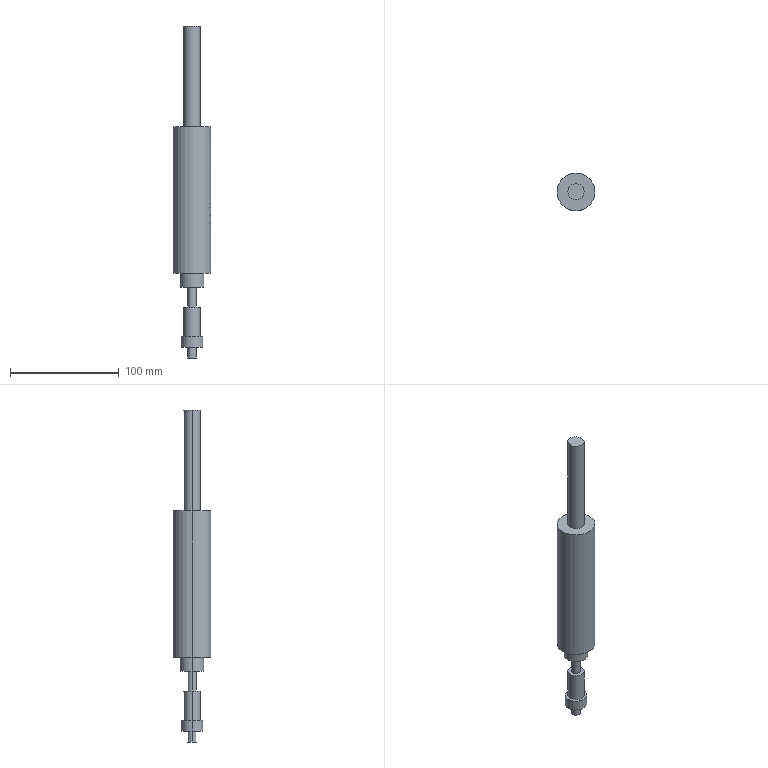Part | 2 solids | 73 faces | box 35 x 35 x 306 mm | volume 159978 mm3 | cylinder 62 | plane 9 | cone 2 | commonest cylinder face diameters 35 x48 8 x4 15 x4 6.8 x2 20 x2 22 x2